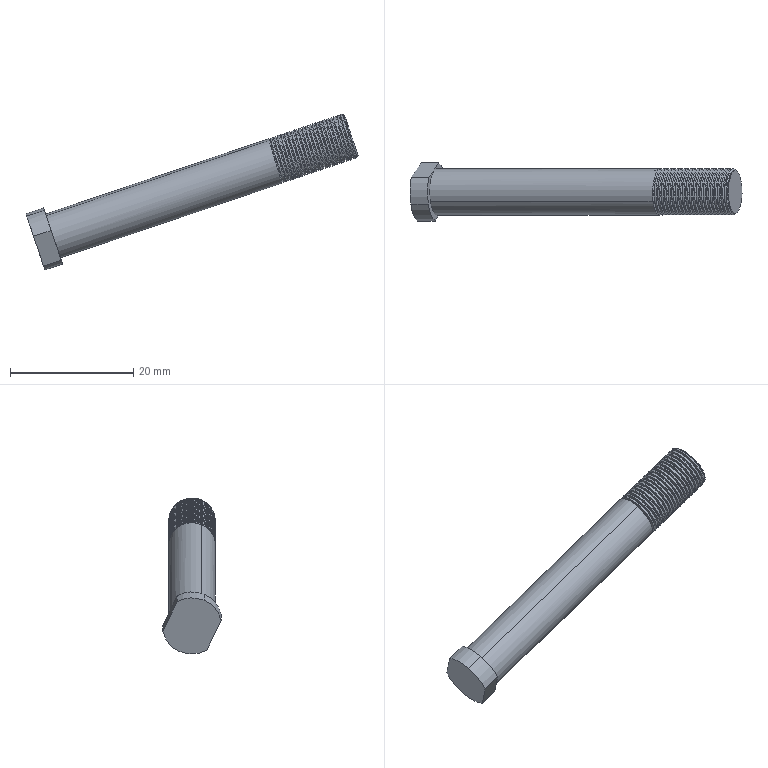Part | STEP file | 2026.6.15-Main Assembly图.sldasm-Part-244 | 1 solid | 60 faces | box 53.801 x 9.404 x 25.282 mm | volume 2422 mm3 | cylinder 48 | plane 6 | spline 3 | cone 3 | commonest cylinder face diameters 7.5 x44 9.6 x4